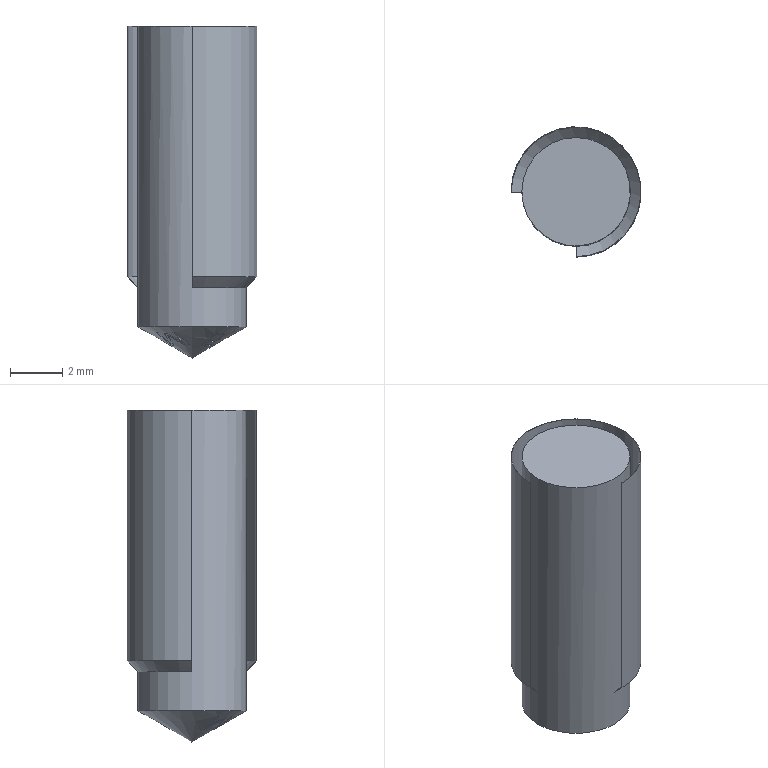Part | STEP file | SOLID | 1 solid | 37 faces | box 5 x 5 x 12.76 mm | volume 163.945 mm3 | plane 24 | cone 5 | other 5 | cylinder 3 | commonest cylinder face diameters 4.167 x1 4.983 x1 5 x1